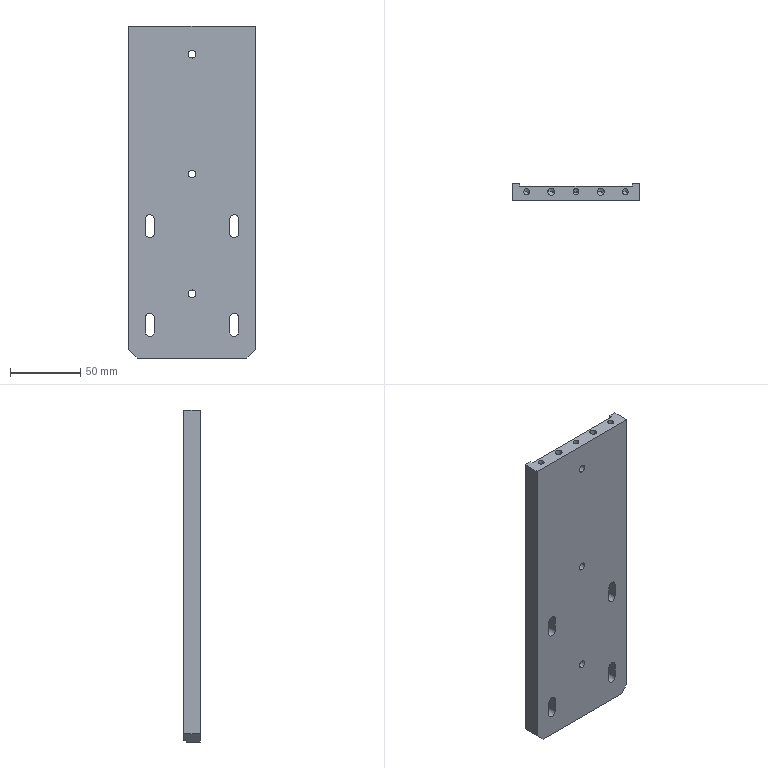Part | STEP file | PN_0056 | 1 solid | 67 faces | box 90 x 12 x 235.5 mm | volume 209838 mm3 | cylinder 34 | plane 23 | cone 10 | commonest cylinder face diameters 6.4 x12 4.2 x6 5.5 x6 10 x6 5 x4